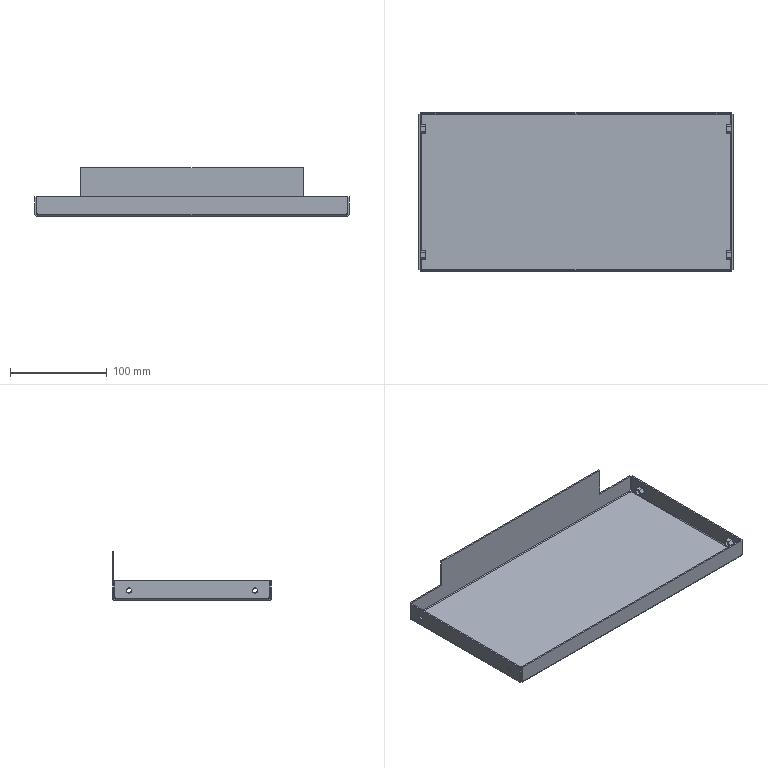Part | SolidWorks | features MoveCopyBody 4, Stock 4, Extrusion 1, FlatPattern 1, FlattenBends 1, ICE 1, ProcessBends 1, Rip 1, SMBaseFlange 1, SheetMetal 1, Shell 1 | 5 solids | 170 faces | box 324 x 164 x 50 mm | volume 116232 mm3 | plane 90 | cone 56 | cylinder 24 | commonest cylinder face diameters 5 x8 5.5 x8 1.5 x4 4.5 x4